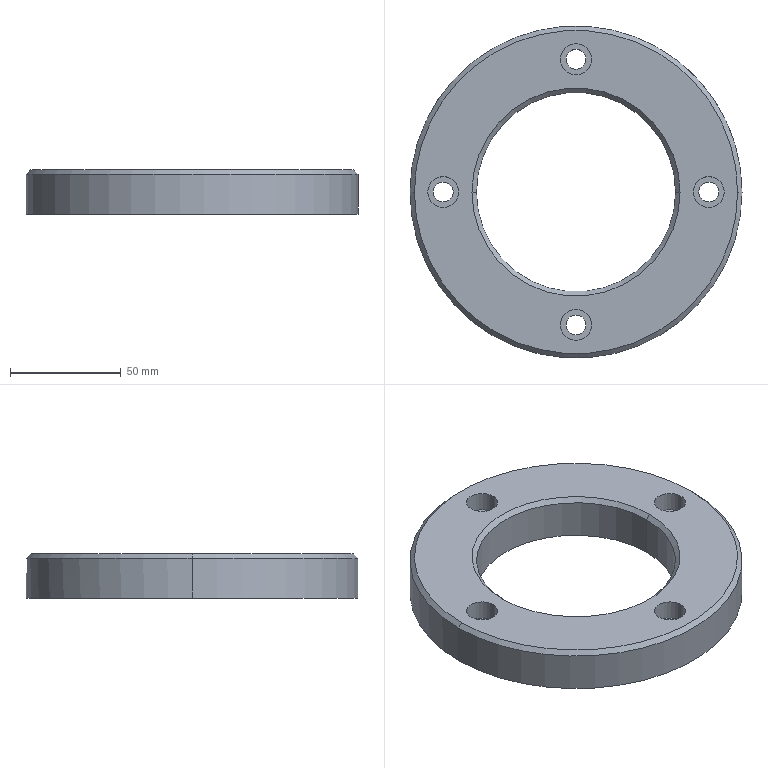Part | Creo | 1 solid | 30 faces | box 150 x 150 x 20 mm | volume 216346 mm3 | cylinder 20 | plane 6 | cone 4 | commonest cylinder face diameters 9 x8 14 x8 90 x2 150 x2
STEP:
#1=CARTESIAN_POINT('',(53.033,53.033,185.5));
#2=VERTEX_POINT('',#1);
#3=CARTESIAN_POINT('',(75.,0.,185.5));
#4=VERTEX_POINT('',#3);
#5=CARTESIAN_POINT('',(0.,0.,185.5));
#6=DIRECTION('',(0.,0.,-1.));
#7=DIRECTION('',(0.7071,0.7071,0.));
#8=AXIS2_PLACEMENT_3D('',#5,#6,#7);
#9=CIRCLE('',#8,75.);
#10=EDGE_CURVE('',#2,#4,#9,.T.);
#11=ORIENTED_EDGE('',*,*,#10,.F.);
#12=CARTESIAN_POINT('',(-75.,0.,185.5));
#13=VERTEX_POINT('',#12);
#14=CARTESIAN_POINT('',(0.,0.,185.5));
#15=DIRECTION('',(0.,0.,-1.));
#16=DIRECTION('',(-1.,0.,0.));
#17=AXIS2_PLACEMENT_3D('',#14,#15,#16);
#18=CIRCLE('',#17,75.);
#19=EDGE_CURVE('',#13,#2,#18,.T.);
#20=ORIENTED_EDGE('',*,*,#19,.F.);
#21=CARTESIAN_POINT('',(0.,0.,185.5));
#22=DIRECTION('',(0.,0.,-1.));
#23=DIRECTION('',(1.,0.,0.));
#24=AXIS2_PLACEMENT_3D('',#21,#22,#23);
#25=CIRCLE('',#24,75.);
#26=EDGE_CURVE('',#4,#13,#25,.T.);
#27=ORIENTED_EDGE('',*,*,#26,.F.);
#28=EDGE_LOOP('',(#11,#20,#27));
#29=FACE_OUTER_BOUND('',#28,.F.);
#30=CARTESIAN_POINT('',(4.5,-60.,185.5));
#31=VERTEX_POINT('',#30);
#32=CARTESIAN_POINT('',(-4.5,-60.,185.5));
#33=VERTEX_POINT('',#32);
#34=CARTESIAN_POINT('',(0.,-60.,185.5));
#35=DIRECTION('',(0.,0.,1.));
#36=DIRECTION('',(1.,0.,0.));
#37=AXIS2_PLACEMENT_3D('',#34,#35,#36);
#38=CIRCLE('',#37,4.5);
#39=EDGE_CURVE('',#31,#33,#38,.T.);
#40=ORIENTED_EDGE('',*,*,#39,.F.);
#41=CARTESIAN_POINT('',(0.,-60.,185.5));
#42=DIRECTION('',(0.,0.,1.));
#43=DIRECTION('',(-1.,0.,0.));
#44=AXIS2_PLACEMENT_3D('',#41,#42,#43);
#45=CIRCLE('',#44,4.5);
#46=EDGE_CURVE('',#33,#31,#45,.T.);
#47=ORIENTED_EDGE('',*,*,#46,.F.);
#48=EDGE_LOOP('',(#40,#47));
#49=FACE_BOUND('',#48,.F.);
#50=CARTESIAN_POINT('',(45.,0.,185.5));
#51=VERTEX_POINT('',#50);
#52=CARTESIAN_POINT('',(-45.,0.,185.5));
#53=VERTEX_POINT('',#52);
#54=CARTESIAN_POINT('',(0.,0.,185.5));
#55=DIRECTION('',(0.,0.,1.));
#56=DIRECTION('',(1.,0.,0.));
#57=AXIS2_PLACEMENT_3D('',#54,#55,#56);
#58=CIRCLE('',#57,45.);
#59=EDGE_CURVE('',#51,#53,#58,.T.);
#60=ORIENTED_EDGE('',*,*,#59,.F.);
#61=CARTESIAN_POINT('',(0.,0.,185.5));
#62=DIRECTION('',(0.,0.,1.));
#63=DIRECTION('',(-1.,0.,0.));
#64=AXIS2_PLACEMENT_3D('',#61,#62,#63);
#65=CIRCLE('',#64,45.);
#66=EDGE_CURVE('',#53,#51,#65,.T.);
#67=ORIENTED_EDGE('',*,*,#66,.F.);
#68=EDGE_LOOP('',(#60,#67));
#69=FACE_BOUND('',#68,.F.);
#70=CARTESIAN_POINT('',(64.5,0.,185.5));
#71=VERTEX_POINT('',#70);
#72=CARTESIAN_POINT('',(55.5,0.,185.5));
#73=VERTEX_POINT('',#72);
#74=CARTESIAN_POINT('',(60.,0.,185.5));
#75=DIRECTION('',(0.,0.,1.));
#76=DIRECTION('',(1.,0.,0.));
#77=AXIS2_PLACEMENT_3D('',#74,#75,#76);
#78=CIRCLE('',#77,4.5);
#79=EDGE_CURVE('',#71,#73,#78,.T.);
#80=ORIENTED_EDGE('',*,*,#79,.F.);
#81=CARTESIAN_POINT('',(60.,0.,185.5));
#82=DIRECTION('',(0.,0.,1.));
#83=DIRECTION('',(-1.,0.,0.));
#84=AXIS2_PLACEMENT_3D('',#81,#82,#83);
#85=CIRCLE('',#84,4.5);
#86=EDGE_CURVE('',#73,#71,#85,.T.);
#87=ORIENTED_EDGE('',*,*,#86,.F.);
#88=EDGE_LOOP('',(#80,#87));
#89=FACE_BOUND('',#88,.F.);
#90=CARTESIAN_POINT('',(-55.5,0.,185.5));
#91=VERTEX_POINT('',#90);
#92=CARTESIAN_POINT('',(-64.5,0.,185.5));
#93=VERTEX_POINT('',#92);
#94=CARTESIAN_POINT('',(-60.,0.,185.5));
#95=DIRECTION('',(0.,0.,1.));
#96=DIRECTION('',(1.,0.,0.));
#97=AXIS2_PLACEMENT_3D('',#94,#95,#96);
#98=CIRCLE('',#97,4.5);
#99=EDGE_CURVE('',#91,#93,#98,.T.);
#100=ORIENTED_EDGE('',*,*,#99,.F.);
#101=CARTESIAN_POINT('',(-60.,0.,185.5));
#102=DIRECTION('',(0.,0.,1.));
#103=DIRECTION('',(-1.,0.,0.));
#104=AXIS2_PLACEMENT_3D('',#101,#102,#103);
#105=CIRCLE('',#104,4.5);
#106=EDGE_CURVE('',#93,#91,#105,.T.);
#107=ORIENTED_EDGE('',*,*,#106,.F.);
#108=EDGE_LOOP('',(#100,#107));
#109=FACE_BOUND('',#108,.F.);
#110=CARTESIAN_POINT('',(4.5,60.,185.5));
#111=VERTEX_POINT('',#110);
#112=CARTESIAN_POINT('',(-4.5,60.,185.5));
#113=VERTEX_POINT('',#112);
#114=CARTESIAN_POINT('',(0.,60.,185.5));
#115=DIRECTION('',(0.,0.,1.));
#116=DIRECTION('',(1.,0.,0.));
#117=AXIS2_PLACEMENT_3D('',#114,#115,#116);
#118=CIRCLE('',#117,4.5);
#119=EDGE_CURVE('',#111,#113,#118,.T.);
#120=ORIENTED_EDGE('',*,*,#119,.F.);
#121=CARTESIAN_POINT('',(0.,60.,185.5));
#122=DIRECTION('',(0.,0.,1.));
#123=DIRECTION('',(-1.,0.,0.));
#124=AXIS2_PLACEMENT_3D('',#121,#122,#123);
#125=CIRCLE('',#124,4.5);
#126=EDGE_CURVE('',#113,#111,#125,.T.);
#127=ORIENTED_EDGE('',*,*,#126,.F.);
#128=EDGE_LOOP('',(#120,#127));
#129=FACE_BOUND('',#128,.F.);
#130=CARTESIAN_POINT('',(0.,0.,185.5));
#131=DIRECTION('',(0.,0.,1.));
#132=DIRECTION('',(1.,0.,0.));
#133=AXIS2_PLACEMENT_3D('',#130,#131,#132);
#134=PLANE('',#133);
#135=ADVANCED_FACE('',(#29,#49,#69,#89,#109,#129),#134,.F.);
#136=CARTESIAN_POINT('',(55.5,0.,196.5));
#137=VERTEX_POINT('',#136);
#138=CARTESIAN_POINT('',(64.5,0.,196.5));
#139=VERTEX_POINT('',#138);
#140=CARTESIAN_POINT('',(60.,0.,196.5));
#141=DIRECTION('',(0.,0.,-1.));
#142=DIRECTION('',(-1.,0.,0.));
#143=AXIS2_PLACEMENT_3D('',#140,#141,#142);
#144=CIRCLE('',#143,4.5);
#145=EDGE_CURVE('',#137,#139,#144,.T.);
#146=ORIENTED_EDGE('',*,*,#145,.T.);
#147=CARTESIAN_POINT('',(64.5,0.,185.5));
#148=DIRECTION('',(0.,0.,1.));
#149=VECTOR('',#148,11.);
#150=LINE('',#147,#149);
#151=EDGE_CURVE('',#71,#139,#150,.T.);
#152=ORIENTED_EDGE('',*,*,#151,.F.);
#153=ORIENTED_EDGE('',*,*,#79,.T.);
#154=CARTESIAN_POINT('',(55.5,0.,185.5));
#155=DIRECTION('',(0.,0.,1.));
#156=VECTOR('',#155,11.);
#157=LINE('',#154,#156);
#158=EDGE_CURVE('',#73,#137,#157,.T.);
#159=ORIENTED_EDGE('',*,*,#158,.T.);
#160=EDGE_LOOP('',(#146,#152,#153,#159));
#161=FACE_OUTER_BOUND('',#160,.F.);
#162=CARTESIAN_POINT('',(60.,0.,185.5));
#163=DIRECTION('',(0.,0.,1.));
#164=DIRECTION('',(1.,0.,0.));
#165=AXIS2_PLACEMENT_3D('',#162,#163,#164);
#166=CYLINDRICAL_SURFACE('',#165,4.5);
#167=ADVANCED_FACE('',(#161),#166,.F.);
#168=CARTESIAN_POINT('',(67.,0.,196.5));
#169=VERTEX_POINT('',#168);
#170=CARTESIAN_POINT('',(53.,0.,196.5));
#171=VERTEX_POINT('',#170);
#172=CARTESIAN_POINT('',(60.,0.,196.5));
#173=DIRECTION('',(0.,0.,1.));
#174=DIRECTION('',(1.,0.,0.));
#175=AXIS2_PLACEMENT_3D('',#172,#173,#174);
#176=CIRCLE('',#175,7.);
#177=EDGE_CURVE('',#169,#171,#176,.T.);
#178=ORIENTED_EDGE('',*,*,#177,.F.);
#179=CARTESIAN_POINT('',(60.,0.,196.5));
#180=DIRECTION('',(0.,0.,1.));
#181=DIRECTION('',(-1.,0.,0.));
#182=AXIS2_PLACEMENT_3D('',#179,#180,#181);
#183=CIRCLE('',#182,7.);
#184=EDGE_CURVE('',#171,#169,#183,.T.);
#185=ORIENTED_EDGE('',*,*,#184,.F.);
#186=EDGE_LOOP('',(#178,#185));
#187=FACE_OUTER_BOUND('',#186,.F.);
#188=CARTESIAN_POINT('',(60.,0.,196.5));
#189=DIRECTION('',(0.,0.,-1.));
#190=DIRECTION('',(1.,0.,0.));
#191=AXIS2_PLACEMENT_3D('',#188,#189,#190);
#192=CIRCLE('',#191,4.5);
#193=EDGE_CURVE('',#139,#137,#192,.T.);
#194=ORIENTED_EDGE('',*,*,#193,.F.);
#195=ORIENTED_EDGE('',*,*,#145,.F.);
#196=EDGE_LOOP('',(#194,#195));
#197=FACE_BOUND('',#196,.F.);
#198=CARTESIAN_POINT('',(60.,0.,196.5));
#199=DIRECTION('',(0.,0.,-1.));
#200=DIRECTION('',(-1.,0.,0.));
#201=AXIS2_PLACEMENT_3D('',#198,#199,#200);
#202=PLANE('',#201);
#203=ADVANCED_FACE('',(#187,#197),#202,.F.);
#204=ORIENTED_EDGE('',*,*,#193,.T.);
#205=ORIENTED_EDGE('',*,*,#158,.F.);
#206=ORIENTED_EDGE('',*,*,#86,.T.);
#207=ORIENTED_EDGE('',*,*,#151,.T.);
#208=EDGE_LOOP('',(#204,#205,#206,#207));
#209=FACE_OUTER_BOUND('',#208,.F.);
#210=CARTESIAN_POINT('',(60.,0.,185.5));
#211=DIRECTION('',(0.,0.,1.));
#212=DIRECTION('',(1.,0.,0.));
#213=AXIS2_PLACEMENT_3D('',#210,#211,#212);
#214=CYLINDRICAL_SURFACE('',#213,4.5);
#215=ADVANCED_FACE('',(#209),#214,.F.);
#216=CARTESIAN_POINT('',(53.,0.,205.5));
#217=VERTEX_POINT('',#216);
#218=CARTESIAN_POINT('',(67.,0.,205.5));
#219=VERTEX_POINT('',#218);
#220=CARTESIAN_POINT('',(60.,0.,205.5));
#221=DIRECTION('',(0.,0.,-1.));
#222=DIRECTION('',(-1.,0.,0.));
#223=AXIS2_PLACEMENT_3D('',#220,#221,#222);
#224=CIRCLE('',#223,7.);
#225=EDGE_CURVE('',#217,#219,#224,.T.);
#226=ORIENTED_EDGE('',*,*,#225,.T.);
#227=CARTESIAN_POINT('',(67.,0.,196.5));
#228=DIRECTION('',(0.,0.,1.));
#229=VECTOR('',#228,9.);
#230=LINE('',#227,#229);
#231=EDGE_CURVE('',#169,#219,#230,.T.);
#232=ORIENTED_EDGE('',*,*,#231,.F.);
#233=ORIENTED_EDGE('',*,*,#177,.T.);
#234=CARTESIAN_POINT('',(53.,0.,196.5));
#235=DIRECTION('',(0.,0.,1.));
#236=VECTOR('',#235,9.);
#237=LINE('',#234,#236);
#238=EDGE_CURVE('',#171,#217,#237,.T.);
#239=ORIENTED_EDGE('',*,*,#238,.T.);
#240=EDGE_LOOP('',(#226,#232,#233,#239));
#241=FACE_OUTER_BOUND('',#240,.F.);
#242=CARTESIAN_POINT('',(60.,0.,196.5));
#243=DIRECTION('',(0.,0.,1.));
#244=DIRECTION('',(1.,0.,0.));
#245=AXIS2_PLACEMENT_3D('',#242,#243,#244);
#246=CYLINDRICAL_SURFACE('',#245,7.);
#247=ADVANCED_FACE('',(#241),#246,.F.);
#248=CARTESIAN_POINT('',(73.,0.,205.5));
#249=VERTEX_POINT('',#248);
#250=CARTESIAN_POINT('',(-73.,0.,205.5));
#251=VERTEX_POINT('',#250);
#252=CARTESIAN_POINT('',(0.,0.,205.5));
#253=DIRECTION('',(0.,0.,1.));
#254=DIRECTION('',(1.,0.,0.));
#255=AXIS2_PLACEMENT_3D('',#252,#253,#254);
#256=CIRCLE('',#255,73.);
#257=EDGE_CURVE('',#249,#251,#256,.T.);
#258=ORIENTED_EDGE('',*,*,#257,.F.);
#259=CARTESIAN_POINT('',(0.,0.,205.5));
#260=DIRECTION('',(0.,0.,1.));
#261=DIRECTION('',(-1.,0.,0.));
#262=AXIS2_PLACEMENT_3D('',#259,#260,#261);
#263=CIRCLE('',#262,73.);
#264=EDGE_CURVE('',#251,#249,#263,.T.);
#265=ORIENTED_EDGE('',*,*,#264,.F.);
#266=EDGE_LOOP('',(#258,#265));
#267=FACE_OUTER_BOUND('',#266,.F.);
#268=CARTESIAN_POINT('',(7.,60.,205.5));
#269=VERTEX_POINT('',#268);
#270=CARTESIAN_POINT('',(-7.,60.,205.5));
#271=VERTEX_POINT('',#270);
#272=CARTESIAN_POINT('',(0.,60.,205.5));
#273=DIRECTION('',(0.,0.,-1.));
#274=DIRECTION('',(1.,0.,0.));
#275=AXIS2_PLACEMENT_3D('',#272,#273,#274);
#276=CIRCLE('',#275,7.);
#277=EDGE_CURVE('',#269,#271,#276,.T.);
#278=ORIENTED_EDGE('',*,*,#277,.F.);
#279=CARTESIAN_POINT('',(0.,60.,205.5));
#280=DIRECTION('',(0.,0.,-1.));
#281=DIRECTION('',(-1.,0.,0.));
#282=AXIS2_PLACEMENT_3D('',#279,#280,#281);
#283=CIRCLE('',#282,7.);
#284=EDGE_CURVE('',#271,#269,#283,.T.);
#285=ORIENTED_EDGE('',*,*,#284,.F.);
#286=EDGE_LOOP('',(#278,#285));
#287=FACE_BOUND('',#286,.F.);
#288=CARTESIAN_POINT('',(7.,-60.,205.5));
#289=VERTEX_POINT('',#288);
#290=CARTESIAN_POINT('',(-7.,-60.,205.5));
#291=VERTEX_POINT('',#290);
#292=CARTESIAN_POINT('',(0.,-60.,205.5));
#293=DIRECTION('',(0.,0.,-1.));
#294=DIRECTION('',(1.,0.,0.));
#295=AXIS2_PLACEMENT_3D('',#292,#293,#294);
#296=CIRCLE('',#295,7.);
#297=EDGE_CURVE('',#289,#291,#296,.T.);
#298=ORIENTED_EDGE('',*,*,#297,.F.);
#299=CARTESIAN_POINT('',(0.,-60.,205.5));
#300=DIRECTION('',(0.,0.,-1.));
#301=DIRECTION('',(-1.,0.,0.));
#302=AXIS2_PLACEMENT_3D('',#299,#300,#301);
#303=CIRCLE('',#302,7.);
#304=EDGE_CURVE('',#291,#289,#303,.T.);
#305=ORIENTED_EDGE('',*,*,#304,.F.);
#306=EDGE_LOOP('',(#298,#305));
#307=FACE_BOUND('',#306,.F.);
#308=CARTESIAN_POINT('',(-53.,0.,205.5));
#309=VERTEX_POINT('',#308);
#310=CARTESIAN_POINT('',(-67.,0.,205.5));
#311=VERTEX_POINT('',#310);
#312=CARTESIAN_POINT('',(-60.,0.,205.5));
#313=DIRECTION('',(0.,0.,-1.));
#314=DIRECTION('',(1.,0.,0.));
#315=AXIS2_PLACEMENT_3D('',#312,#313,#314);
#316=CIRCLE('',#315,7.);
#317=EDGE_CURVE('',#309,#311,#316,.T.);
#318=ORIENTED_EDGE('',*,*,#317,.F.);
#319=CARTESIAN_POINT('',(-60.,0.,205.5));
#320=DIRECTION('',(0.,0.,-1.));
#321=DIRECTION('',(-1.,0.,0.));
#322=AXIS2_PLACEMENT_3D('',#319,#320,#321);
#323=CIRCLE('',#322,7.);
#324=EDGE_CURVE('',#311,#309,#323,.T.);
#325=ORIENTED_EDGE('',*,*,#324,.F.);
#326=EDGE_LOOP('',(#318,#325));
#327=FACE_BOUND('',#326,.F.);
#328=CARTESIAN_POINT('',(47.,0.,205.5));
#329=VERTEX_POINT('',#328);
#330=CARTESIAN_POINT('',(-47.,0.,205.5));
#331=VERTEX_POINT('',#330);
#332=CARTESIAN_POINT('',(0.,0.,205.5));
#333=DIRECTION('',(0.,0.,-1.));
#334=DIRECTION('',(1.,0.,0.));
#335=AXIS2_PLACEMENT_3D('',#332,#333,#334);
#336=CIRCLE('',#335,47.);
#337=EDGE_CURVE('',#329,#331,#336,.T.);
#338=ORIENTED_EDGE('',*,*,#337,.F.);
#339=CARTESIAN_POINT('',(0.,0.,205.5));
#340=DIRECTION('',(0.,0.,-1.));
#341=DIRECTION('',(-1.,0.,0.));
#342=AXIS2_PLACEMENT_3D('',#339,#340,#341);
#343=CIRCLE('',#342,47.);
#344=EDGE_CURVE('',#331,#329,#343,.T.);
#345=ORIENTED_EDGE('',*,*,#344,.F.);
#346=EDGE_LOOP('',(#338,#345));
#347=FACE_BOUND('',#346,.F.);
#348=CARTESIAN_POINT('',(60.,0.,205.5));
#349=DIRECTION('',(0.,0.,-1.));
#350=DIRECTION('',(1.,0.,0.));
#351=AXIS2_PLACEMENT_3D('',#348,#349,#350);
#352=CIRCLE('',#351,7.);
#353=EDGE_CURVE('',#219,#217,#352,.T.);
#354=ORIENTED_EDGE('',*,*,#353,.F.);
#355=ORIENTED_EDGE('',*,*,#225,.F.);
#356=EDGE_LOOP('',(#354,#355));
#357=FACE_BOUND('',#356,.F.);
#358=CARTESIAN_POINT('',(0.,0.,205.5));
#359=DIRECTION('',(0.,0.,1.));
#360=DIRECTION('',(1.,0.,0.));
#361=AXIS2_PLACEMENT_3D('',#358,#359,#360);
#362=PLANE('',#361);
#363=ADVANCED_FACE('',(#267,#287,#307,#327,#347,#357),#362,.T.);
#364=ORIENTED_EDGE('',*,*,#353,.T.);
#365=ORIENTED_EDGE('',*,*,#238,.F.);
#366=ORIENTED_EDGE('',*,*,#184,.T.);
#367=ORIENTED_EDGE('',*,*,#231,.T.);
#368=EDGE_LOOP('',(#364,#365,#366,#367));
#369=FACE_OUTER_BOUND('',#368,.F.);
#370=CARTESIAN_POINT('',(60.,0.,196.5));
#371=DIRECTION('',(0.,0.,1.));
#372=DIRECTION('',(1.,0.,0.));
#373=AXIS2_PLACEMENT_3D('',#370,#371,#372);
#374=CYLINDRICAL_SURFACE('',#373,7.);
#375=ADVANCED_FACE('',(#369),#374,.F.);
#376=ORIENTED_EDGE('',*,*,#277,.T.);
#377=CARTESIAN_POINT('',(-7.,60.,196.5));
#378=VERTEX_POINT('',#377);
#379=CARTESIAN_POINT('',(-7.,60.,196.5));
#380=DIRECTION('',(0.,0.,1.));
#381=VECTOR('',#380,9.);
#382=LINE('',#379,#381);
#383=EDGE_CURVE('',#378,#271,#382,.T.);
#384=ORIENTED_EDGE('',*,*,#383,.F.);
#385=CARTESIAN_POINT('',(7.,60.,196.5));
#386=VERTEX_POINT('',#385);
#387=CARTESIAN_POINT('',(0.,60.,196.5));
#388=DIRECTION('',(0.,0.,1.));
#389=DIRECTION('',(-1.,0.,0.));
#390=AXIS2_PLACEMENT_3D('',#387,#388,#389);
#391=CIRCLE('',#390,7.);
#392=EDGE_CURVE('',#378,#386,#391,.T.);
#393=ORIENTED_EDGE('',*,*,#392,.T.);
#394=CARTESIAN_POINT('',(7.,60.,196.5));
#395=DIRECTION('',(0.,0.,1.));
#396=VECTOR('',#395,9.);
#397=LINE('',#394,#396);
#398=EDGE_CURVE('',#386,#269,#397,.T.);
#399=ORIENTED_EDGE('',*,*,#398,.T.);
#400=EDGE_LOOP('',(#376,#384,#393,#399));
#401=FACE_OUTER_BOUND('',#400,.F.);
#402=CARTESIAN_POINT('',(0.,60.,196.5));
#403=DIRECTION('',(0.,0.,1.));
#404=DIRECTION('',(1.,0.,0.));
#405=AXIS2_PLACEMENT_3D('',#402,#403,#404);
#406=CYLINDRICAL_SURFACE('',#405,7.);
#407=ADVANCED_FACE('',(#401),#406,.F.);
#408=ORIENTED_EDGE('',*,*,#284,.T.);
#409=ORIENTED_EDGE('',*,*,#398,.F.);
#410=CARTESIAN_POINT('',(0.,60.,196.5));
#411=DIRECTION('',(0.,0.,1.));
#412=DIRECTION('',(1.,0.,0.));
#413=AXIS2_PLACEMENT_3D('',#410,#411,#412);
#414=CIRCLE('',#413,7.);
#415=EDGE_CURVE('',#386,#378,#414,.T.);
#416=ORIENTED_EDGE('',*,*,#415,.T.);
#417=ORIENTED_EDGE('',*,*,#383,.T.);
#418=EDGE_LOOP('',(#408,#409,#416,#417));
#419=FACE_OUTER_BOUND('',#418,.F.);
#420=CARTESIAN_POINT('',(0.,60.,196.5));
#421=DIRECTION('',(0.,0.,1.));
#422=DIRECTION('',(1.,0.,0.));
#423=AXIS2_PLACEMENT_3D('',#420,#421,#422);
#424=CYLINDRICAL_SURFACE('',#423,7.);
#425=ADVANCED_FACE('',(#419),#424,.F.);
#426=ORIENTED_EDGE('',*,*,#415,.F.);
#427=ORIENTED_EDGE('',*,*,#392,.F.);
#428=EDGE_LOOP('',(#426,#427));
#429=FACE_OUTER_BOUND('',#428,.F.);
#430=CARTESIAN_POINT('',(4.5,60.,196.5));
#431=VERTEX_POINT('',#430);
#432=CARTESIAN_POINT('',(-4.5,60.,196.5));
#433=VERTEX_POINT('',#432);
#434=CARTESIAN_POINT('',(0.,60.,196.5));
#435=DIRECTION('',(0.,0.,-1.));
#436=DIRECTION('',(1.,0.,0.));
#437=AXIS2_PLACEMENT_3D('',#434,#435,#436);
#438=CIRCLE('',#437,4.5);
#439=EDGE_CURVE('',#431,#433,#438,.T.);
#440=ORIENTED_EDGE('',*,*,#439,.F.);
#441=CARTESIAN_POINT('',(0.,60.,196.5));
#442=DIRECTION('',(0.,0.,-1.));
#443=DIRECTION('',(-1.,0.,0.));
#444=AXIS2_PLACEMENT_3D('',#441,#442,#443);
#445=CIRCLE('',#444,4.5);
#446=EDGE_CURVE('',#433,#431,#445,.T.);
#447=ORIENTED_EDGE('',*,*,#446,.F.);
#448=EDGE_LOOP('',(#440,#447));
#449=FACE_BOUND('',#448,.F.);
#450=CARTESIAN_POINT('',(0.,60.,196.5));
#451=DIRECTION('',(0.,0.,-1.));
#452=DIRECTION('',(-1.,0.,0.));
#453=AXIS2_PLACEMENT_3D('',#450,#451,#452);
#454=PLANE('',#453);
#455=ADVANCED_FACE('',(#429,#449),#454,.F.);
#456=ORIENTED_EDGE('',*,*,#439,.T.);
#457=CARTESIAN_POINT('',(-4.5,60.,185.5));
#458=DIRECTION('',(0.,0.,1.));
#459=VECTOR('',#458,11.);
#460=LINE('',#457,#459);
#461=EDGE_CURVE('',#113,#433,#460,.T.);
#462=ORIENTED_EDGE('',*,*,#461,.F.);
#463=ORIENTED_EDGE('',*,*,#126,.T.);
#464=CARTESIAN_POINT('',(4.5,60.,185.5));
#465=DIRECTION('',(0.,0.,1.));
#466=VECTOR('',#465,11.);
#467=LINE('',#464,#466);
#468=EDGE_CURVE('',#111,#431,#467,.T.);
#469=ORIENTED_EDGE('',*,*,#468,.T.);
#470=EDGE_LOOP('',(#456,#462,#463,#469));
#471=FACE_OUTER_BOUND('',#470,.F.);
#472=CARTESIAN_POINT('',(0.,60.,185.5));
#473=DIRECTION('',(0.,0.,1.));
#474=DIRECTION('',(1.,0.,0.));
#475=AXIS2_PLACEMENT_3D('',#472,#473,#474);
#476=CYLINDRICAL_SURFACE('',#475,4.5);
#477=ADVANCED_FACE('',(#471),#476,.F.);
#478=ORIENTED_EDGE('',*,*,#446,.T.);
#479=ORIENTED_EDGE('',*,*,#468,.F.);
#480=ORIENTED_EDGE('',*,*,#119,.T.);
#481=ORIENTED_EDGE('',*,*,#461,.T.);
#482=EDGE_LOOP('',(#478,#479,#480,#481));
#483=FACE_OUTER_BOUND('',#482,.F.);
#484=CARTESIAN_POINT('',(0.,60.,185.5));
#485=DIRECTION('',(0.,0.,1.));
#486=DIRECTION('',(1.,0.,0.));
#487=AXIS2_PLACEMENT_3D('',#484,#485,#486);
#488=CYLINDRICAL_SURFACE('',#487,4.5);
#489=ADVANCED_FACE('',(#483),#488,.F.);
#490=ORIENTED_EDGE('',*,*,#297,.T.);
#491=CARTESIAN_POINT('',(-7.,-60.,196.5));
#492=VERTEX_POINT('',#491);
#493=CARTESIAN_POINT('',(-7.,-60.,196.5));
#494=DIRECTION('',(0.,0.,1.));
#495=VECTOR('',#494,9.);
#496=LINE('',#493,#495);
#497=EDGE_CURVE('',#492,#291,#496,.T.);
#498=ORIENTED_EDGE('',*,*,#497,.F.);
#499=CARTESIAN_POINT('',(7.,-60.,196.5));
#500=VERTEX_POINT('',#499);
#501=CARTESIAN_POINT('',(0.,-60.,196.5));
#502=DIRECTION('',(0.,0.,1.));
#503=DIRECTION('',(-1.,0.,0.));
#504=AXIS2_PLACEMENT_3D('',#501,#502,#503);
#505=CIRCLE('',#504,7.);
#506=EDGE_CURVE('',#492,#500,#505,.T.);
#507=ORIENTED_EDGE('',*,*,#506,.T.);
#508=CARTESIAN_POINT('',(7.,-60.,196.5));
#509=DIRECTION('',(0.,0.,1.));
#510=VECTOR('',#509,9.);
#511=LINE('',#508,#510);
#512=EDGE_CURVE('',#500,#289,#511,.T.);
#513=ORIENTED_EDGE('',*,*,#512,.T.);
#514=EDGE_LOOP('',(#490,#498,#507,#513));
#515=FACE_OUTER_BOUND('',#514,.F.);
#516=CARTESIAN_POINT('',(0.,-60.,196.5));
#517=DIRECTION('',(0.,0.,1.));
#518=DIRECTION('',(1.,0.,0.));
#519=AXIS2_PLACEMENT_3D('',#516,#517,#518);
#520=CYLINDRICAL_SURFACE('',#519,7.);
#521=ADVANCED_FACE('',(#515),#520,.F.);
#522=ORIENTED_EDGE('',*,*,#304,.T.);
#523=ORIENTED_EDGE('',*,*,#512,.F.);
#524=CARTESIAN_POINT('',(0.,-60.,196.5));
#525=DIRECTION('',(0.,0.,1.));
#526=DIRECTION('',(1.,0.,0.));
#527=AXIS2_PLACEMENT_3D('',#524,#525,#526);
#528=CIRCLE('',#527,7.);
#529=EDGE_CURVE('',#500,#492,#528,.T.);
#530=ORIENTED_EDGE('',*,*,#529,.T.);
#531=ORIENTED_EDGE('',*,*,#497,.T.);
#532=EDGE_LOOP('',(#522,#523,#530,#531));
#533=FACE_OUTER_BOUND('',#532,.F.);
#534=CARTESIAN_POINT('',(0.,-60.,196.5));
#535=DIRECTION('',(0.,0.,1.));
#536=DIRECTION('',(1.,0.,0.));
#537=AXIS2_PLACEMENT_3D('',#534,#535,#536);
#538=CYLINDRICAL_SURFACE('',#537,7.);
#539=ADVANCED_FACE('',(#533),#538,.F.);
#540=ORIENTED_EDGE('',*,*,#529,.F.);
#541=ORIENTED_EDGE('',*,*,#506,.F.);
#542=EDGE_LOOP('',(#540,#541));
#543=FACE_OUTER_BOUND('',#542,.F.);
#544=CARTESIAN_POINT('',(4.5,-60.,196.5));
#545=VERTEX_POINT('',#544);
#546=CARTESIAN_POINT('',(-4.5,-60.,196.5));
#547=VERTEX_POINT('',#546);
#548=CARTESIAN_POINT('',(0.,-60.,196.5));
#549=DIRECTION('',(0.,0.,-1.));
#550=DIRECTION('',(1.,0.,0.));
#551=AXIS2_PLACEMENT_3D('',#548,#549,#550);
#552=CIRCLE('',#551,4.5);
#553=EDGE_CURVE('',#545,#547,#552,.T.);
#554=ORIENTED_EDGE('',*,*,#553,.F.);
#555=CARTESIAN_POINT('',(0.,-60.,196.5));
#556=DIRECTION('',(0.,0.,-1.));
#557=DIRECTION('',(-1.,0.,0.));
#558=AXIS2_PLACEMENT_3D('',#555,#556,#557);
#559=CIRCLE('',#558,4.5);
#560=EDGE_CURVE('',#547,#545,#559,.T.);
#561=ORIENTED_EDGE('',*,*,#560,.F.);
#562=EDGE_LOOP('',(#554,#561));
#563=FACE_BOUND('',#562,.F.);
#564=CARTESIAN_POINT('',(0.,-60.,196.5));
#565=DIRECTION('',(0.,0.,-1.));
#566=DIRECTION('',(-1.,0.,0.));
#567=AXIS2_PLACEMENT_3D('',#564,#565,#566);
#568=PLANE('',#567);
#569=ADVANCED_FACE('',(#543,#563),#568,.F.);
#570=ORIENTED_EDGE('',*,*,#553,.T.);
#571=CARTESIAN_POINT('',(-4.5,-60.,185.5));
#572=DIRECTION('',(0.,0.,1.));
#573=VECTOR('',#572,11.);
#574=LINE('',#571,#573);
#575=EDGE_CURVE('',#33,#547,#574,.T.);
#576=ORIENTED_EDGE('',*,*,#575,.F.);
#577=ORIENTED_EDGE('',*,*,#46,.T.);
#578=CARTESIAN_POINT('',(4.5,-60.,185.5));
#579=DIRECTION('',(0.,0.,1.));
#580=VECTOR('',#579,11.);
#581=LINE('',#578,#580);
#582=EDGE_CURVE('',#31,#545,#581,.T.);
#583=ORIENTED_EDGE('',*,*,#582,.T.);
#584=EDGE_LOOP('',(#570,#576,#577,#583));
#585=FACE_OUTER_BOUND('',#584,.F.);
#586=CARTESIAN_POINT('',(0.,-60.,185.5));
#587=DIRECTION('',(0.,0.,1.));
#588=DIRECTION('',(1.,0.,0.));
#589=AXIS2_PLACEMENT_3D('',#586,#587,#588);
#590=CYLINDRICAL_SURFACE('',#589,4.5);
#591=ADVANCED_FACE('',(#585),#590,.F.);
#592=ORIENTED_EDGE('',*,*,#560,.T.);
#593=ORIENTED_EDGE('',*,*,#582,.F.);
#594=ORIENTED_EDGE('',*,*,#39,.T.);
#595=ORIENTED_EDGE('',*,*,#575,.T.);
#596=EDGE_LOOP('',(#592,#593,#594,#595));
#597=FACE_OUTER_BOUND('',#596,.F.);
#598=CARTESIAN_POINT('',(0.,-60.,185.5));
#599=DIRECTION('',(0.,0.,1.));
#600=DIRECTION('',(1.,0.,0.));
#601=AXIS2_PLACEMENT_3D('',#598,#599,#600);
#602=CYLINDRICAL_SURFACE('',#601,4.5);
#603=ADVANCED_FACE('',(#597),#602,.F.);
#604=ORIENTED_EDGE('',*,*,#317,.T.);
#605=CARTESIAN_POINT('',(-67.,0.,196.5));
#606=VERTEX_POINT('',#605);
#607=CARTESIAN_POINT('',(-67.,0.,196.5));
#608=DIRECTION('',(0.,0.,1.));
#609=VECTOR('',#608,9.);
#610=LINE('',#607,#609);
#611=EDGE_CURVE('',#606,#311,#610,.T.);
#612=ORIENTED_EDGE('',*,*,#611,.F.);
#613=CARTESIAN_POINT('',(-53.,0.,196.5));
#614=VERTEX_POINT('',#613);
#615=CARTESIAN_POINT('',(-60.,0.,196.5));
#616=DIRECTION('',(0.,0.,1.));
#617=DIRECTION('',(-1.,0.,0.));
#618=AXIS2_PLACEMENT_3D('',#615,#616,#617);
#619=CIRCLE('',#618,7.);
#620=EDGE_CURVE('',#606,#614,#619,.T.);
#621=ORIENTED_EDGE('',*,*,#620,.T.);
#622=CARTESIAN_POINT('',(-53.,0.,196.5));
#623=DIRECTION('',(0.,0.,1.));
#624=VECTOR('',#623,9.);
#625=LINE('',#622,#624);
#626=EDGE_CURVE('',#614,#309,#625,.T.);
#627=ORIENTED_EDGE('',*,*,#626,.T.);
#628=EDGE_LOOP('',(#604,#612,#621,#627));
#629=FACE_OUTER_BOUND('',#628,.F.);
#630=CARTESIAN_POINT('',(-60.,0.,196.5));
#631=DIRECTION('',(0.,0.,1.));
#632=DIRECTION('',(1.,0.,0.));
#633=AXIS2_PLACEMENT_3D('',#630,#631,#632);
#634=CYLINDRICAL_SURFACE('',#633,7.);
#635=ADVANCED_FACE('',(#629),#634,.F.);
#636=ORIENTED_EDGE('',*,*,#324,.T.);
#637=ORIENTED_EDGE('',*,*,#626,.F.);
#638=CARTESIAN_POINT('',(-60.,0.,196.5));
#639=DIRECTION('',(0.,0.,1.));
#640=DIRECTION('',(1.,0.,0.));
#641=AXIS2_PLACEMENT_3D('',#638,#639,#640);
#642=CIRCLE('',#641,7.);
#643=EDGE_CURVE('',#614,#606,#642,.T.);
#644=ORIENTED_EDGE('',*,*,#643,.T.);
#645=ORIENTED_EDGE('',*,*,#611,.T.);
#646=EDGE_LOOP('',(#636,#637,#644,#645));
#647=FACE_OUTER_BOUND('',#646,.F.);
#648=CARTESIAN_POINT('',(-60.,0.,196.5));
#649=DIRECTION('',(0.,0.,1.));
#650=DIRECTION('',(1.,0.,0.));
#651=AXIS2_PLACEMENT_3D('',#648,#649,#650);
#652=CYLINDRICAL_SURFACE('',#651,7.);
#653=ADVANCED_FACE('',(#647),#652,.F.);
#654=ORIENTED_EDGE('',*,*,#643,.F.);
#655=ORIENTED_EDGE('',*,*,#620,.F.);
#656=EDGE_LOOP('',(#654,#655));
#657=FACE_OUTER_BOUND('',#656,.F.);
#658=CARTESIAN_POINT('',(-55.5,0.,196.5));
#659=VERTEX_POINT('',#658);
#660=CARTESIAN_POINT('',(-64.5,0.,196.5));
#661=VERTEX_POINT('',#660);
#662=CARTESIAN_POINT('',(-60.,0.,196.5));
#663=DIRECTION('',(0.,0.,-1.));
#664=DIRECTION('',(1.,0.,0.));
#665=AXIS2_PLACEMENT_3D('',#662,#663,#664);
#666=CIRCLE('',#665,4.5);
#667=EDGE_CURVE('',#659,#661,#666,.T.);
#668=ORIENTED_EDGE('',*,*,#667,.F.);
#669=CARTESIAN_POINT('',(-60.,0.,196.5));
#670=DIRECTION('',(0.,0.,-1.));
#671=DIRECTION('',(-1.,0.,0.));
#672=AXIS2_PLACEMENT_3D('',#669,#670,#671);
#673=CIRCLE('',#672,4.5);
#674=EDGE_CURVE('',#661,#659,#673,.T.);
#675=ORIENTED_EDGE('',*,*,#674,.F.);
#676=EDGE_LOOP('',(#668,#675));
#677=FACE_BOUND('',#676,.F.);
#678=CARTESIAN_POINT('',(-60.,0.,196.5));
#679=DIRECTION('',(0.,0.,-1.));
#680=DIRECTION('',(-1.,0.,0.));
#681=AXIS2_PLACEMENT_3D('',#678,#679,#680);
#682=PLANE('',#681);
#683=ADVANCED_FACE('',(#657,#677),#682,.F.);
#684=ORIENTED_EDGE('',*,*,#667,.T.);
#685=CARTESIAN_POINT('',(-64.5,0.,185.5));
#686=DIRECTION('',(0.,0.,1.));
#687=VECTOR('',#686,11.);
#688=LINE('',#685,#687);
#689=EDGE_CURVE('',#93,#661,#688,.T.);
#690=ORIENTED_EDGE('',*,*,#689,.F.);
#691=ORIENTED_EDGE('',*,*,#106,.T.);
#692=CARTESIAN_POINT('',(-55.5,0.,185.5));
#693=DIRECTION('',(0.,0.,1.));
#694=VECTOR('',#693,11.);
#695=LINE('',#692,#694);
#696=EDGE_CURVE('',#91,#659,#695,.T.);
#697=ORIENTED_EDGE('',*,*,#696,.T.);
#698=EDGE_LOOP('',(#684,#690,#691,#697));
#699=FACE_OUTER_BOUND('',#698,.F.);
#700=CARTESIAN_POINT('',(-60.,0.,185.5));
#701=DIRECTION('',(0.,0.,1.));
#702=DIRECTION('',(1.,0.,0.));
#703=AXIS2_PLACEMENT_3D('',#700,#701,#702);
#704=CYLINDRICAL_SURFACE('',#703,4.5);
#705=ADVANCED_FACE('',(#699),#704,.F.);
#706=ORIENTED_EDGE('',*,*,#674,.T.);
#707=ORIENTED_EDGE('',*,*,#696,.F.);
#708=ORIENTED_EDGE('',*,*,#99,.T.);
#709=ORIENTED_EDGE('',*,*,#689,.T.);
#710=EDGE_LOOP('',(#706,#707,#708,#709));
#711=FACE_OUTER_BOUND('',#710,.F.);
#712=CARTESIAN_POINT('',(-60.,0.,185.5));
#713=DIRECTION('',(0.,0.,1.));
#714=DIRECTION('',(1.,0.,0.));
#715=AXIS2_PLACEMENT_3D('',#712,#713,#714);
#716=CYLINDRICAL_SURFACE('',#715,4.5);
#717=ADVANCED_FACE('',(#711),#716,.F.);
#718=CARTESIAN_POINT('',(45.,0.,203.5));
#719=VERTEX_POINT('',#718);
#720=CARTESIAN_POINT('',(-45.,0.,203.5));
#721=VERTEX_POINT('',#720);
#722=CARTESIAN_POINT('',(0.,0.,203.5));
#723=DIRECTION('',(0.,0.,-1.));
#724=DIRECTION('',(1.,0.,0.));
#725=AXIS2_PLACEMENT_3D('',#722,#723,#724);
#726=CIRCLE('',#725,45.);
#727=EDGE_CURVE('',#719,#721,#726,.T.);
#728=ORIENTED_EDGE('',*,*,#727,.F.);
#729=CARTESIAN_POINT('',(45.,0.,203.5));
#730=DIRECTION('',(0.7071,0.,0.7071));
#731=VECTOR('',#730,2.828);
#732=LINE('',#729,#731);
#733=EDGE_CURVE('',#719,#329,#732,.T.);
#734=ORIENTED_EDGE('',*,*,#733,.T.);
#735=ORIENTED_EDGE('',*,*,#337,.T.);
#736=CARTESIAN_POINT('',(-45.,0.,203.5));
#737=DIRECTION('',(-0.7071,0.,0.7071));
#738=VECTOR('',#737,2.828);
#739=LINE('',#736,#738);
#740=EDGE_CURVE('',#721,#331,#739,.T.);
#741=ORIENTED_EDGE('',*,*,#740,.F.);
#742=EDGE_LOOP('',(#728,#734,#735,#741));
#743=FACE_OUTER_BOUND('',#742,.F.);
#744=CARTESIAN_POINT('',(0.,0.,204.5));
#745=DIRECTION('',(0.,0.,1.));
#746=DIRECTION('',(1.,0.,0.));
#747=AXIS2_PLACEMENT_3D('',#744,#745,#746);
#748=CONICAL_SURFACE('',#747,46.,45.);
#749=ADVANCED_FACE('',(#743),#748,.F.);
#750=ORIENTED_EDGE('',*,*,#727,.T.);
#751=CARTESIAN_POINT('',(-45.,0.,203.5));
#752=DIRECTION('',(0.,0.,-1.));
#753=VECTOR('',#752,18.);
#754=LINE('',#751,#753);
#755=EDGE_CURVE('',#721,#53,#754,.T.);
#756=ORIENTED_EDGE('',*,*,#755,.T.);
#757=ORIENTED_EDGE('',*,*,#66,.T.);
#758=CARTESIAN_POINT('',(45.,0.,203.5));
#759=DIRECTION('',(0.,0.,-1.));
#760=VECTOR('',#759,18.);
#761=LINE('',#758,#760);
#762=EDGE_CURVE('',#719,#51,#761,.T.);
#763=ORIENTED_EDGE('',*,*,#762,.F.);
#764=EDGE_LOOP('',(#750,#756,#757,#763));
#765=FACE_OUTER_BOUND('',#764,.F.);
#766=CARTESIAN_POINT('',(0.,0.,205.5));
#767=DIRECTION('',(0.,0.,-1.));
#768=DIRECTION('',(-1.,0.,0.));
#769=AXIS2_PLACEMENT_3D('',#766,#767,#768);
#770=CYLINDRICAL_SURFACE('',#769,45.);
#771=ADVANCED_FACE('',(#765),#770,.F.);
#772=CARTESIAN_POINT('',(0.,0.,203.5));
#773=DIRECTION('',(0.,0.,-1.));
#774=DIRECTION('',(-1.,0.,0.));
#775=AXIS2_PLACEMENT_3D('',#772,#773,#774);
#776=CIRCLE('',#775,45.);
#777=EDGE_CURVE('',#721,#719,#776,.T.);
#778=ORIENTED_EDGE('',*,*,#777,.T.);
#779=ORIENTED_EDGE('',*,*,#762,.T.);
#780=ORIENTED_EDGE('',*,*,#59,.T.);
#781=ORIENTED_EDGE('',*,*,#755,.F.);
#782=EDGE_LOOP('',(#778,#779,#780,#781));
#783=FACE_OUTER_BOUND('',#782,.F.);
#784=CARTESIAN_POINT('',(0.,0.,205.5));
#785=DIRECTION('',(0.,0.,-1.));
#786=DIRECTION('',(-1.,0.,0.));
#787=AXIS2_PLACEMENT_3D('',#784,#785,#786);
#788=CYLINDRICAL_SURFACE('',#787,45.);
#789=ADVANCED_FACE('',(#783),#788,.F.);
#790=ORIENTED_EDGE('',*,*,#777,.F.);
#791=ORIENTED_EDGE('',*,*,#740,.T.);
#792=ORIENTED_EDGE('',*,*,#344,.T.);
#793=ORIENTED_EDGE('',*,*,#733,.F.);
#794=EDGE_LOOP('',(#790,#791,#792,#793));
#795=FACE_OUTER_BOUND('',#794,.F.);
#796=CARTESIAN_POINT('',(0.,0.,204.5));
#797=DIRECTION('',(0.,0.,1.));
#798=DIRECTION('',(1.,0.,0.));
#799=AXIS2_PLACEMENT_3D('',#796,#797,#798);
#800=CONICAL_SURFACE('',#799,46.,45.);
#801=ADVANCED_FACE('',(#795),#800,.F.);
#802=CARTESIAN_POINT('',(75.,0.,203.5));
#803=VERTEX_POINT('',#802);
#804=CARTESIAN_POINT('',(-75.,0.,203.5));
#805=VERTEX_POINT('',#804);
#806=CARTESIAN_POINT('',(0.,0.,203.5));
#807=DIRECTION('',(0.,0.,1.));
#808=DIRECTION('',(1.,0.,0.));
#809=AXIS2_PLACEMENT_3D('',#806,#807,#808);
#810=CIRCLE('',#809,75.);
#811=EDGE_CURVE('',#803,#805,#810,.T.);
#812=ORIENTED_EDGE('',*,*,#811,.F.);
#813=CARTESIAN_POINT('',(73.,0.,205.5));
#814=DIRECTION('',(0.7071,0.,-0.7071));
#815=VECTOR('',#814,2.828);
#816=LINE('',#813,#815);
#817=EDGE_CURVE('',#249,#803,#816,.T.);
#818=ORIENTED_EDGE('',*,*,#817,.F.);
#819=ORIENTED_EDGE('',*,*,#257,.T.);
#820=CARTESIAN_POINT('',(-73.,0.,205.5));
#821=DIRECTION('',(-0.7071,0.,-0.7071));
#822=VECTOR('',#821,2.828);
#823=LINE('',#820,#822);
#824=EDGE_CURVE('',#251,#805,#823,.T.);
#825=ORIENTED_EDGE('',*,*,#824,.T.);
#826=EDGE_LOOP('',(#812,#818,#819,#825));
#827=FACE_OUTER_BOUND('',#826,.F.);
#828=CARTESIAN_POINT('',(0.,0.,204.5));
#829=DIRECTION('',(0.,0.,-1.));
#830=DIRECTION('',(-1.,0.,0.));
#831=AXIS2_PLACEMENT_3D('',#828,#829,#830);
#832=CONICAL_SURFACE('',#831,74.,45.);
#833=ADVANCED_FACE('',(#827),#832,.T.);
#834=ORIENTED_EDGE('',*,*,#811,.T.);
#835=CARTESIAN_POINT('',(-75.,0.,203.5));
#836=DIRECTION('',(0.,0.,-1.));
#837=VECTOR('',#836,18.);
#838=LINE('',#835,#837);
#839=EDGE_CURVE('',#805,#13,#838,.T.);
#840=ORIENTED_EDGE('',*,*,#839,.T.);
#841=ORIENTED_EDGE('',*,*,#19,.T.);
#842=ORIENTED_EDGE('',*,*,#10,.T.);
#843=CARTESIAN_POINT('',(75.,0.,203.5));
#844=DIRECTION('',(0.,0.,-1.));
#845=VECTOR('',#844,18.);
#846=LINE('',#843,#845);
#847=EDGE_CURVE('',#803,#4,#846,.T.);
#848=ORIENTED_EDGE('',*,*,#847,.F.);
#849=EDGE_LOOP('',(#834,#840,#841,#842,#848));
#850=FACE_OUTER_BOUND('',#849,.F.);
#851=CARTESIAN_POINT('',(0.,0.,205.5));
#852=DIRECTION('',(0.,0.,-1.));
#853=DIRECTION('',(-1.,0.,0.));
#854=AXIS2_PLACEMENT_3D('',#851,#852,#853);
#855=CYLINDRICAL_SURFACE('',#854,75.);
#856=ADVANCED_FACE('',(#850),#855,.T.);
#857=CARTESIAN_POINT('',(0.,0.,203.5));
#858=DIRECTION('',(0.,0.,1.));
#859=DIRECTION('',(-1.,0.,0.));
#860=AXIS2_PLACEMENT_3D('',#857,#858,#859);
#861=CIRCLE('',#860,75.);
#862=EDGE_CURVE('',#805,#803,#861,.T.);
#863=ORIENTED_EDGE('',*,*,#862,.T.);
#864=ORIENTED_EDGE('',*,*,#847,.T.);
#865=ORIENTED_EDGE('',*,*,#26,.T.);
#866=ORIENTED_EDGE('',*,*,#839,.F.);
#867=EDGE_LOOP('',(#863,#864,#865,#866));
#868=FACE_OUTER_BOUND('',#867,.F.);
#869=CARTESIAN_POINT('',(0.,0.,205.5));
#870=DIRECTION('',(0.,0.,-1.));
#871=DIRECTION('',(-1.,0.,0.));
#872=AXIS2_PLACEMENT_3D('',#869,#870,#871);
#873=CYLINDRICAL_SURFACE('',#872,75.);
#874=ADVANCED_FACE('',(#868),#873,.T.);
#875=ORIENTED_EDGE('',*,*,#862,.F.);
#876=ORIENTED_EDGE('',*,*,#824,.F.);
#877=ORIENTED_EDGE('',*,*,#264,.T.);
#878=ORIENTED_EDGE('',*,*,#817,.T.);
#879=EDGE_LOOP('',(#875,#876,#877,#878));
#880=FACE_OUTER_BOUND('',#879,.F.);
#881=CARTESIAN_POINT('',(0.,0.,204.5));
#882=DIRECTION('',(0.,0.,-1.));
#883=DIRECTION('',(-1.,0.,0.));
#884=AXIS2_PLACEMENT_3D('',#881,#882,#883);
#885=CONICAL_SURFACE('',#884,74.,45.);
#886=ADVANCED_FACE('',(#880),#885,.T.);
#887=CLOSED_SHELL('',(#135,#167,#203,#215,#247,#363,#375,#407,#425,#455,#477,#489,#521,#539,#569,#591,#603,#635,#653,#683,#705,#717,#749,#771,#789,#801,#833,#856,#874,#886));
#888=MANIFOLD_SOLID_BREP('',#887);
#889=(LENGTH_UNIT()NAMED_UNIT(*)SI_UNIT(.MILLI.,.METRE.));
#890=UNCERTAINTY_MEASURE_WITH_UNIT(LENGTH_MEASURE(0.02131),#889,'','');
#891=(NAMED_UNIT(*)PLANE_ANGLE_UNIT()SI_UNIT($,.RADIAN.));
#892=PLANE_ANGLE_MEASURE_WITH_UNIT(PLANE_ANGLE_MEASURE(0.01745),#891);
#893=(CONVERSION_BASED_UNIT('DEGREE',#892)NAMED_UNIT(*)PLANE_ANGLE_UNIT());
#894=(NAMED_UNIT(*)SI_UNIT($,.STERADIAN.)SOLID_ANGLE_UNIT());
#895=(GEOMETRIC_REPRESENTATION_CONTEXT(3)GLOBAL_UNCERTAINTY_ASSIGNED_CONTEXT((#890))GLOBAL_UNIT_ASSIGNED_CONTEXT((#889,#893,#894))REPRESENTATION_CONTEXT('',''));
#896=ADVANCED_BREP_SHAPE_REPRESENTATION('',(#888),#895);